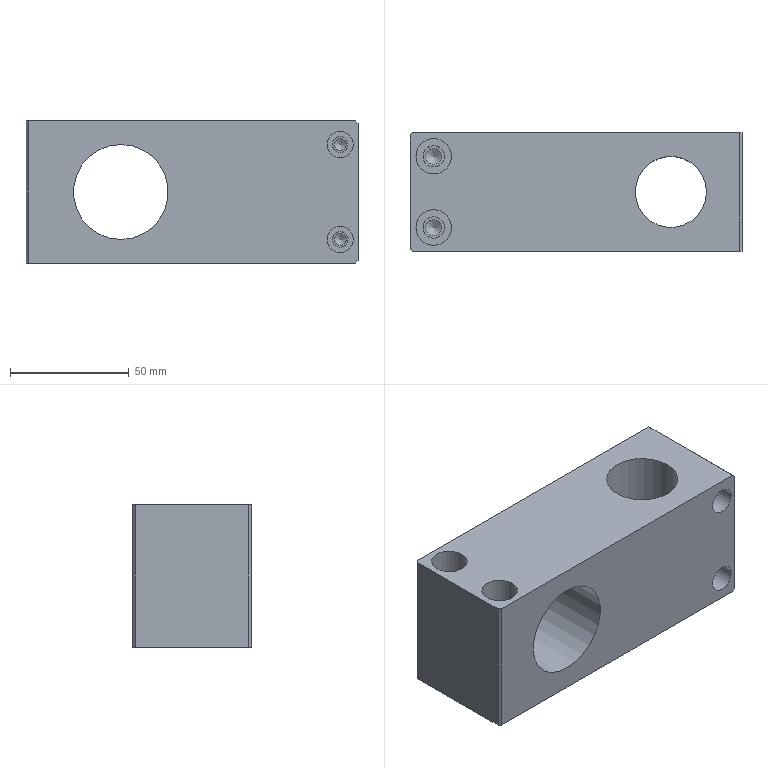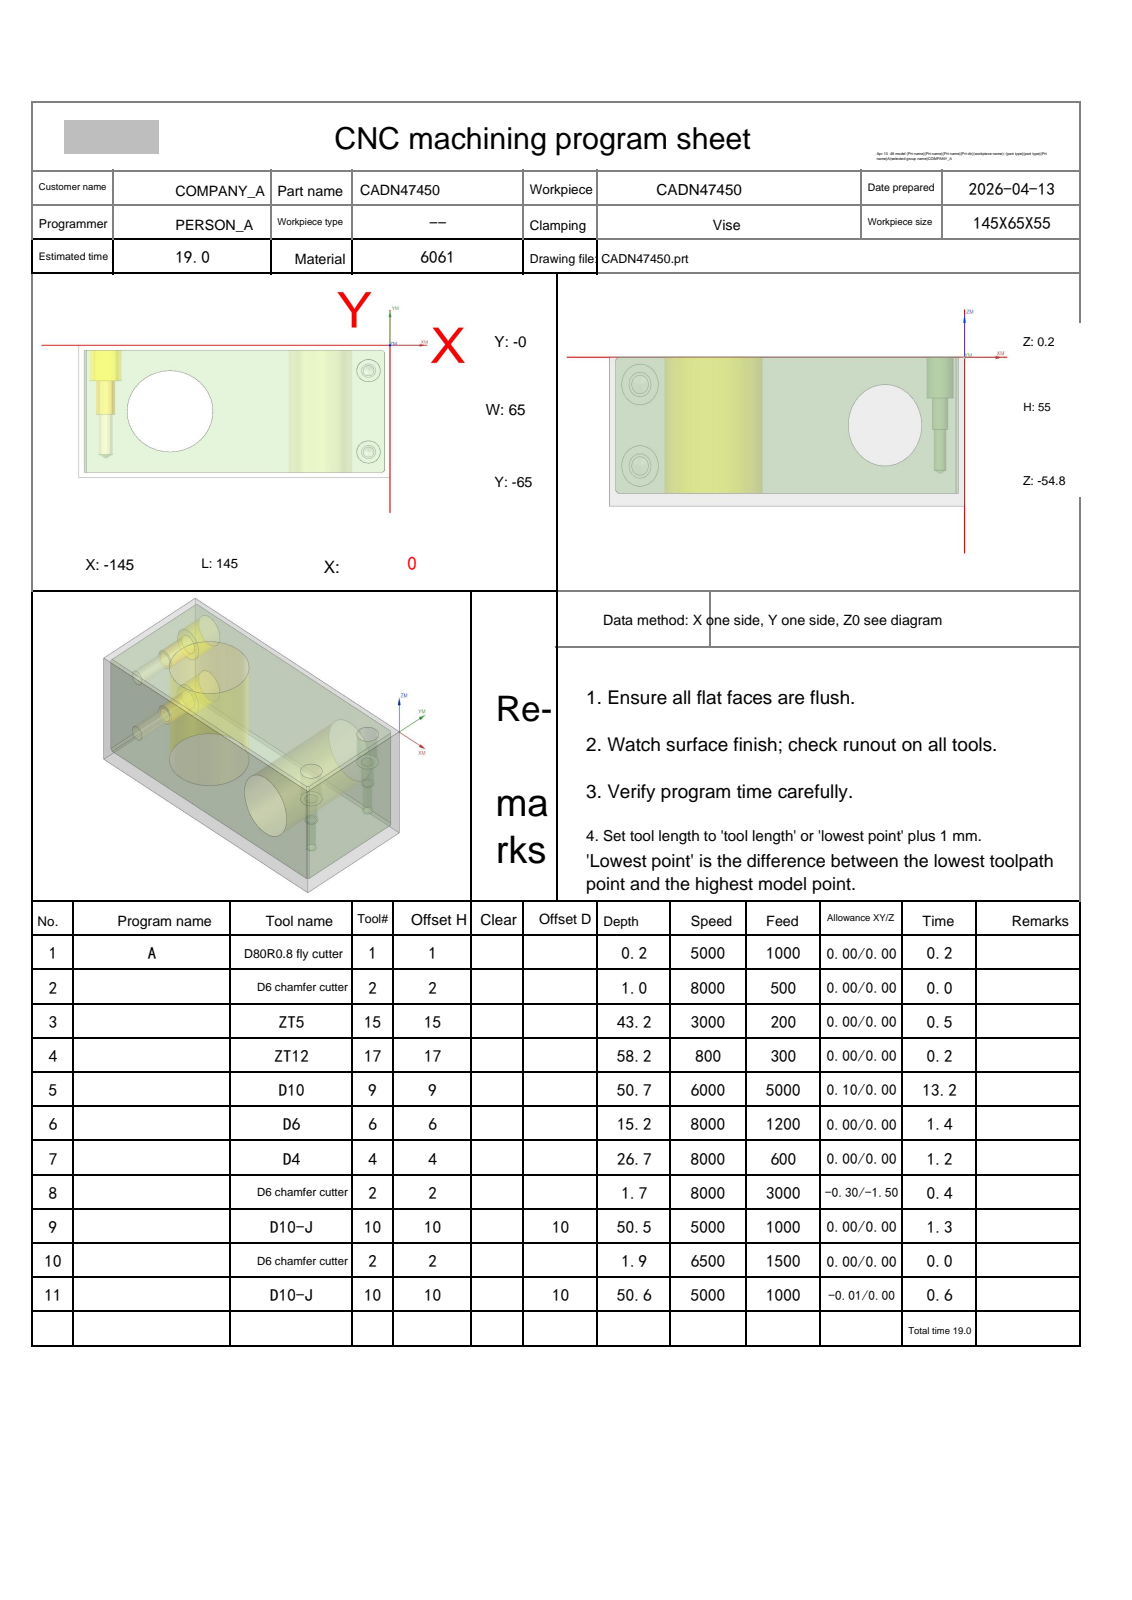NC program | NX | posted by the shop | part box 140 x 50 x 60 mm
Lines 1 to 76 of 4750:
%
O0001
(Machine time: 21.32 MIN)
(===Total Tool:8===)
(T1=D80R0.8 fly cutter D=80.  R=0.8  D-  H01 Z=0.    )
(T2=D6 chamfer cutter   D=6.   R=0.   D-  H02 Z=-1.7  )
(T15=ZT5    D=5.   DR_a=118 D-  H15 Z=-43.  )
(T17=ZT12   D=12.  DR_a=118 D-  H17 Z=-58.  )
(T9=D10     D=10.  R=0.   D-  H09 Z=-50.5 )
(T6=D6      D=6.   R=0.   D-  H06 Z=-15.  )
(T4=D4      D=4.   R=0.   D-  H04 Z=-26.5 )
(T10=D10-J  D=10.  R=0.   D10 H10 Z=-50.4 )
G80 G90 G17 G49 G40
G91 G28 Z0
M01
N1 T01 M06
(D80R0.8 fly cutter  D=80. R=0.8 H=01 ce=0.00 di=0.00)
G00 G90 G54 X42.5 Y-32.5 M03 S5000
G43 H01 Z20.
M08
Z2.
G01 Z0.0 F1000.
X37.5
X-182.5
X-187.5
Z2.
G00 Z20.
G91 G28 Z0.0
M05
M09
G91 G28 Z0.0
M01
N2 T02 M06
(D6 chamfer cutter  D=6. R=0. H=02 ce=0.00 di=0.00)
G00 G90 G54 X-10. Y-52.5 M03 S8000
G43 H02 Z20.
M08
G98 G81 X-10. Y-52.5 Z-.8 R1. F500.
Y-12.5
X-102.5 Y-32.5
G80
G00 Z20.
G91 G28 Z0.0
M05
M09
G91 G28 Z0.0
M01
N3 T15 M06
(ZT5 D=5. DR_a=118 H=15)
G00 G90 G54 X-10. Y-52.5 M03 S3000
G43 H15 Z20.
M08
G98 G83 X-10. Y-52.5 Z-43.002 R1. F200. Q2.
Y-12.5
G80
G00 Z20.
G91 G28 Z0.0
M05
M09
G91 G28 Z0.0
M01
N4 T17 M06
(ZT12 D=12. DR_a=118 H=17)
G00 G90 G54 X-102.5 Y-32.5 M03 S800
G43 H17 Z20.
M08
G98 G83 X-102.5 Y-32.5 Z-58. R1. F300. Q3.
G80
G00 Z20.
G91 G28 Z0.0
M05
M09
G91 G28 Z0.0
M01